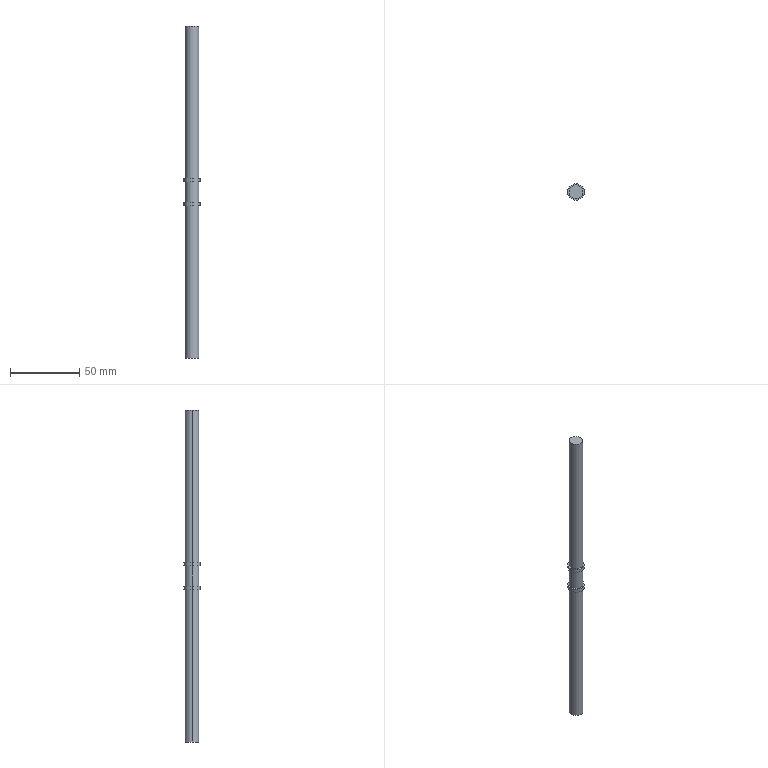Part | STEP file | Adjusting lead screw QY-1-16 | 1 solid | 16 faces | box 12 x 12 x 240 mm | volume 19022 mm3 | cylinder 10 | plane 6 | commonest cylinder face diameters 10 x6 12 x4
STEP:
#1=CARTESIAN_POINT('',(0.,0.,0.));
#2=DIRECTION('',(0.,0.,1.));
#3=DIRECTION('',(1.,0.,0.));
#4=AXIS2_PLACEMENT_3D('',#1,#2,#3);
#5=CARTESIAN_POINT('',(6.,0.,10.));
#6=VERTEX_POINT('',#5);
#7=CARTESIAN_POINT('',(-6.,0.,10.));
#8=VERTEX_POINT('',#7);
#9=CARTESIAN_POINT('',(0.,0.,10.));
#10=DIRECTION('',(0.,0.,1.));
#11=DIRECTION('',(1.,0.,0.));
#12=AXIS2_PLACEMENT_3D('',#9,#10,#11);
#13=CIRCLE('',#12,6.);
#14=CARTESIAN_POINT('',(0.,0.,10.));
#15=DIRECTION('',(0.,0.,-1.));
#16=DIRECTION('',(-1.,0.,0.));
#17=AXIS2_PLACEMENT_3D('',#14,#15,#16);
#18=CYLINDRICAL_SURFACE('',#17,6.);
#19=CARTESIAN_POINT('',(3.142,0.));
#20=DIRECTION('',(-1.,0.));
#21=VECTOR('',#20,1.);
#22=LINE('',#19,#21);
#23=(GEOMETRIC_REPRESENTATION_CONTEXT(2)PARAMETRIC_REPRESENTATION_CONTEXT()REPRESENTATION_CONTEXT('',''));
#24=DEFINITIONAL_REPRESENTATION('',(#22),#23);
#25=PCURVE('',#18,#24);
#26=CARTESIAN_POINT('',(0.,0.,10.));
#27=DIRECTION('',(0.,0.,1.));
#28=DIRECTION('',(1.,0.,0.));
#29=AXIS2_PLACEMENT_3D('',#26,#27,#28);
#30=PLANE('',#29);
#31=CARTESIAN_POINT('',(0.,0.));
#32=DIRECTION('',(1.,0.));
#33=AXIS2_PLACEMENT_2D('',#31,#32);
#34=CIRCLE('',#33,6.);
#35=(GEOMETRIC_REPRESENTATION_CONTEXT(2)PARAMETRIC_REPRESENTATION_CONTEXT()REPRESENTATION_CONTEXT('',''));
#36=DEFINITIONAL_REPRESENTATION('',(#34),#35);
#37=PCURVE('',#30,#36);
#38=SURFACE_CURVE('',#13,(#25,#37),.PCURVE_S1.);
#39=EDGE_CURVE('',#6,#8,#38,.T.);
#40=ORIENTED_EDGE('',*,*,#39,.F.);
#41=CARTESIAN_POINT('',(6.,0.,7.5));
#42=VERTEX_POINT('',#41);
#43=CARTESIAN_POINT('',(6.,0.,10.));
#44=DIRECTION('',(0.,0.,-1.));
#45=VECTOR('',#44,1.);
#46=LINE('',#43,#45);
#47=CARTESIAN_POINT('',(3.142,0.));
#48=DIRECTION('',(0.,1.));
#49=VECTOR('',#48,1.);
#50=LINE('',#47,#49);
#51=(GEOMETRIC_REPRESENTATION_CONTEXT(2)PARAMETRIC_REPRESENTATION_CONTEXT()REPRESENTATION_CONTEXT('',''));
#52=DEFINITIONAL_REPRESENTATION('',(#50),#51);
#53=PCURVE('',#18,#52);
#54=CARTESIAN_POINT('',(0.,0.,10.));
#55=DIRECTION('',(0.,0.,-1.));
#56=DIRECTION('',(-1.,0.,0.));
#57=AXIS2_PLACEMENT_3D('',#54,#55,#56);
#58=CYLINDRICAL_SURFACE('',#57,6.);
#59=CARTESIAN_POINT('',(3.142,0.));
#60=DIRECTION('',(0.,1.));
#61=VECTOR('',#60,1.);
#62=LINE('',#59,#61);
#63=(GEOMETRIC_REPRESENTATION_CONTEXT(2)PARAMETRIC_REPRESENTATION_CONTEXT()REPRESENTATION_CONTEXT('',''));
#64=DEFINITIONAL_REPRESENTATION('',(#62),#63);
#65=PCURVE('',#58,#64);
#66=SURFACE_CURVE('',#46,(#53,#65),.PCURVE_S1.);
#67=EDGE_CURVE('',#6,#42,#66,.T.);
#68=ORIENTED_EDGE('',*,*,#67,.T.);
#69=CARTESIAN_POINT('',(-6.,0.,7.5));
#70=VERTEX_POINT('',#69);
#71=CARTESIAN_POINT('',(0.,0.,7.5));
#72=DIRECTION('',(0.,0.,1.));
#73=DIRECTION('',(1.,0.,0.));
#74=AXIS2_PLACEMENT_3D('',#71,#72,#73);
#75=CIRCLE('',#74,6.);
#76=CARTESIAN_POINT('',(3.142,2.5));
#77=DIRECTION('',(-1.,0.));
#78=VECTOR('',#77,1.);
#79=LINE('',#76,#78);
#80=(GEOMETRIC_REPRESENTATION_CONTEXT(2)PARAMETRIC_REPRESENTATION_CONTEXT()REPRESENTATION_CONTEXT('',''));
#81=DEFINITIONAL_REPRESENTATION('',(#79),#80);
#82=PCURVE('',#18,#81);
#83=CARTESIAN_POINT('',(0.,0.,7.5));
#84=DIRECTION('',(0.,0.,1.));
#85=DIRECTION('',(1.,0.,0.));
#86=AXIS2_PLACEMENT_3D('',#83,#84,#85);
#87=PLANE('',#86);
#88=CARTESIAN_POINT('',(0.,0.));
#89=DIRECTION('',(1.,0.));
#90=AXIS2_PLACEMENT_2D('',#88,#89);
#91=CIRCLE('',#90,6.);
#92=(GEOMETRIC_REPRESENTATION_CONTEXT(2)PARAMETRIC_REPRESENTATION_CONTEXT()REPRESENTATION_CONTEXT('',''));
#93=DEFINITIONAL_REPRESENTATION('',(#91),#92);
#94=PCURVE('',#87,#93);
#95=SURFACE_CURVE('',#75,(#82,#94),.PCURVE_S1.);
#96=EDGE_CURVE('',#42,#70,#95,.T.);
#97=ORIENTED_EDGE('',*,*,#96,.T.);
#98=CARTESIAN_POINT('',(-6.,0.,10.));
#99=DIRECTION('',(0.,0.,-1.));
#100=VECTOR('',#99,1.);
#101=LINE('',#98,#100);
#102=CARTESIAN_POINT('',(0.,0.));
#103=DIRECTION('',(0.,1.));
#104=VECTOR('',#103,1.);
#105=LINE('',#102,#104);
#106=(GEOMETRIC_REPRESENTATION_CONTEXT(2)PARAMETRIC_REPRESENTATION_CONTEXT()REPRESENTATION_CONTEXT('',''));
#107=DEFINITIONAL_REPRESENTATION('',(#105),#106);
#108=PCURVE('',#18,#107);
#109=CARTESIAN_POINT('',(6.283,0.));
#110=DIRECTION('',(0.,1.));
#111=VECTOR('',#110,1.);
#112=LINE('',#109,#111);
#113=(GEOMETRIC_REPRESENTATION_CONTEXT(2)PARAMETRIC_REPRESENTATION_CONTEXT()REPRESENTATION_CONTEXT('',''));
#114=DEFINITIONAL_REPRESENTATION('',(#112),#113);
#115=PCURVE('',#58,#114);
#116=SURFACE_CURVE('',#101,(#108,#115),.PCURVE_S1.);
#117=EDGE_CURVE('',#8,#70,#116,.T.);
#118=ORIENTED_EDGE('',*,*,#117,.F.);
#119=EDGE_LOOP('',(#40,#68,#97,#118));
#120=FACE_BOUND('',#119,.T.);
#121=ADVANCED_FACE('',(#120),#18,.T.);
#122=CARTESIAN_POINT('',(5.,0.,120.));
#123=VERTEX_POINT('',#122);
#124=CARTESIAN_POINT('',(-5.,0.,120.));
#125=VERTEX_POINT('',#124);
#126=CARTESIAN_POINT('',(0.,0.,120.));
#127=DIRECTION('',(0.,0.,1.));
#128=DIRECTION('',(1.,0.,0.));
#129=AXIS2_PLACEMENT_3D('',#126,#127,#128);
#130=CIRCLE('',#129,5.);
#131=CARTESIAN_POINT('',(0.,0.,120.));
#132=DIRECTION('',(0.,0.,-1.));
#133=DIRECTION('',(-1.,0.,0.));
#134=AXIS2_PLACEMENT_3D('',#131,#132,#133);
#135=CYLINDRICAL_SURFACE('',#134,5.);
#136=CARTESIAN_POINT('',(3.142,0.));
#137=DIRECTION('',(-1.,0.));
#138=VECTOR('',#137,1.);
#139=LINE('',#136,#138);
#140=(GEOMETRIC_REPRESENTATION_CONTEXT(2)PARAMETRIC_REPRESENTATION_CONTEXT()REPRESENTATION_CONTEXT('',''));
#141=DEFINITIONAL_REPRESENTATION('',(#139),#140);
#142=PCURVE('',#135,#141);
#143=CARTESIAN_POINT('',(0.,0.,120.));
#144=DIRECTION('',(0.,0.,1.));
#145=DIRECTION('',(1.,0.,0.));
#146=AXIS2_PLACEMENT_3D('',#143,#144,#145);
#147=PLANE('',#146);
#148=CARTESIAN_POINT('',(0.,0.));
#149=DIRECTION('',(1.,0.));
#150=AXIS2_PLACEMENT_2D('',#148,#149);
#151=CIRCLE('',#150,5.);
#152=(GEOMETRIC_REPRESENTATION_CONTEXT(2)PARAMETRIC_REPRESENTATION_CONTEXT()REPRESENTATION_CONTEXT('',''));
#153=DEFINITIONAL_REPRESENTATION('',(#151),#152);
#154=PCURVE('',#147,#153);
#155=SURFACE_CURVE('',#130,(#142,#154),.PCURVE_S1.);
#156=EDGE_CURVE('',#123,#125,#155,.T.);
#157=ORIENTED_EDGE('',*,*,#156,.F.);
#158=CARTESIAN_POINT('',(5.,0.,10.));
#159=VERTEX_POINT('',#158);
#160=CARTESIAN_POINT('',(5.,0.,120.));
#161=DIRECTION('',(0.,0.,-1.));
#162=VECTOR('',#161,1.);
#163=LINE('',#160,#162);
#164=CARTESIAN_POINT('',(3.142,0.));
#165=DIRECTION('',(0.,1.));
#166=VECTOR('',#165,1.);
#167=LINE('',#164,#166);
#168=(GEOMETRIC_REPRESENTATION_CONTEXT(2)PARAMETRIC_REPRESENTATION_CONTEXT()REPRESENTATION_CONTEXT('',''));
#169=DEFINITIONAL_REPRESENTATION('',(#167),#168);
#170=PCURVE('',#135,#169);
#171=CARTESIAN_POINT('',(0.,0.,120.));
#172=DIRECTION('',(0.,0.,-1.));
#173=DIRECTION('',(-1.,0.,0.));
#174=AXIS2_PLACEMENT_3D('',#171,#172,#173);
#175=CYLINDRICAL_SURFACE('',#174,5.);
#176=CARTESIAN_POINT('',(3.142,0.));
#177=DIRECTION('',(0.,1.));
#178=VECTOR('',#177,1.);
#179=LINE('',#176,#178);
#180=(GEOMETRIC_REPRESENTATION_CONTEXT(2)PARAMETRIC_REPRESENTATION_CONTEXT()REPRESENTATION_CONTEXT('',''));
#181=DEFINITIONAL_REPRESENTATION('',(#179),#180);
#182=PCURVE('',#175,#181);
#183=SURFACE_CURVE('',#163,(#170,#182),.PCURVE_S1.);
#184=EDGE_CURVE('',#123,#159,#183,.T.);
#185=ORIENTED_EDGE('',*,*,#184,.T.);
#186=CARTESIAN_POINT('',(-5.,0.,10.));
#187=VERTEX_POINT('',#186);
#188=CARTESIAN_POINT('',(0.,0.,10.));
#189=DIRECTION('',(0.,0.,1.));
#190=DIRECTION('',(1.,0.,0.));
#191=AXIS2_PLACEMENT_3D('',#188,#189,#190);
#192=CIRCLE('',#191,5.);
#193=CARTESIAN_POINT('',(3.142,110.));
#194=DIRECTION('',(-1.,0.));
#195=VECTOR('',#194,1.);
#196=LINE('',#193,#195);
#197=(GEOMETRIC_REPRESENTATION_CONTEXT(2)PARAMETRIC_REPRESENTATION_CONTEXT()REPRESENTATION_CONTEXT('',''));
#198=DEFINITIONAL_REPRESENTATION('',(#196),#197);
#199=PCURVE('',#135,#198);
#200=CARTESIAN_POINT('',(0.,0.));
#201=DIRECTION('',(1.,0.));
#202=AXIS2_PLACEMENT_2D('',#200,#201);
#203=CIRCLE('',#202,5.);
#204=(GEOMETRIC_REPRESENTATION_CONTEXT(2)PARAMETRIC_REPRESENTATION_CONTEXT()REPRESENTATION_CONTEXT('',''));
#205=DEFINITIONAL_REPRESENTATION('',(#203),#204);
#206=PCURVE('',#30,#205);
#207=SURFACE_CURVE('',#192,(#199,#206),.PCURVE_S1.);
#208=EDGE_CURVE('',#159,#187,#207,.T.);
#209=ORIENTED_EDGE('',*,*,#208,.T.);
#210=CARTESIAN_POINT('',(-5.,0.,120.));
#211=DIRECTION('',(0.,0.,-1.));
#212=VECTOR('',#211,1.);
#213=LINE('',#210,#212);
#214=CARTESIAN_POINT('',(0.,0.));
#215=DIRECTION('',(0.,1.));
#216=VECTOR('',#215,1.);
#217=LINE('',#214,#216);
#218=(GEOMETRIC_REPRESENTATION_CONTEXT(2)PARAMETRIC_REPRESENTATION_CONTEXT()REPRESENTATION_CONTEXT('',''));
#219=DEFINITIONAL_REPRESENTATION('',(#217),#218);
#220=PCURVE('',#135,#219);
#221=CARTESIAN_POINT('',(6.283,0.));
#222=DIRECTION('',(0.,1.));
#223=VECTOR('',#222,1.);
#224=LINE('',#221,#223);
#225=(GEOMETRIC_REPRESENTATION_CONTEXT(2)PARAMETRIC_REPRESENTATION_CONTEXT()REPRESENTATION_CONTEXT('',''));
#226=DEFINITIONAL_REPRESENTATION('',(#224),#225);
#227=PCURVE('',#175,#226);
#228=SURFACE_CURVE('',#213,(#220,#227),.PCURVE_S1.);
#229=EDGE_CURVE('',#125,#187,#228,.T.);
#230=ORIENTED_EDGE('',*,*,#229,.F.);
#231=EDGE_LOOP('',(#157,#185,#209,#230));
#232=FACE_BOUND('',#231,.T.);
#233=ADVANCED_FACE('',(#232),#135,.T.);
#234=CARTESIAN_POINT('',(5.,0.,-7.5));
#235=VERTEX_POINT('',#234);
#236=CARTESIAN_POINT('',(-5.,0.,-7.5));
#237=VERTEX_POINT('',#236);
#238=CARTESIAN_POINT('',(0.,0.,-7.5));
#239=DIRECTION('',(0.,0.,1.));
#240=DIRECTION('',(1.,0.,0.));
#241=AXIS2_PLACEMENT_3D('',#238,#239,#240);
#242=CIRCLE('',#241,5.);
#243=CARTESIAN_POINT('',(0.,0.,-7.5));
#244=DIRECTION('',(0.,0.,1.));
#245=DIRECTION('',(1.,0.,0.));
#246=AXIS2_PLACEMENT_3D('',#243,#244,#245);
#247=CYLINDRICAL_SURFACE('',#246,5.);
#248=CARTESIAN_POINT('',(0.,0.));
#249=DIRECTION('',(1.,0.));
#250=VECTOR('',#249,1.);
#251=LINE('',#248,#250);
#252=(GEOMETRIC_REPRESENTATION_CONTEXT(2)PARAMETRIC_REPRESENTATION_CONTEXT()REPRESENTATION_CONTEXT('',''));
#253=DEFINITIONAL_REPRESENTATION('',(#251),#252);
#254=PCURVE('',#247,#253);
#255=CARTESIAN_POINT('',(0.,0.,-7.5));
#256=DIRECTION('',(0.,0.,1.));
#257=DIRECTION('',(1.,0.,0.));
#258=AXIS2_PLACEMENT_3D('',#255,#256,#257);
#259=PLANE('',#258);
#260=CARTESIAN_POINT('',(0.,0.));
#261=DIRECTION('',(1.,0.));
#262=AXIS2_PLACEMENT_2D('',#260,#261);
#263=CIRCLE('',#262,5.);
#264=(GEOMETRIC_REPRESENTATION_CONTEXT(2)PARAMETRIC_REPRESENTATION_CONTEXT()REPRESENTATION_CONTEXT('',''));
#265=DEFINITIONAL_REPRESENTATION('',(#263),#264);
#266=PCURVE('',#259,#265);
#267=SURFACE_CURVE('',#242,(#254,#266),.PCURVE_S1.);
#268=EDGE_CURVE('',#235,#237,#267,.T.);
#269=ORIENTED_EDGE('',*,*,#268,.T.);
#270=CARTESIAN_POINT('',(-5.,0.,7.5));
#271=VERTEX_POINT('',#270);
#272=CARTESIAN_POINT('',(-5.,0.,-7.5));
#273=DIRECTION('',(0.,0.,1.));
#274=VECTOR('',#273,1.);
#275=LINE('',#272,#274);
#276=CARTESIAN_POINT('',(3.142,0.));
#277=DIRECTION('',(0.,1.));
#278=VECTOR('',#277,1.);
#279=LINE('',#276,#278);
#280=(GEOMETRIC_REPRESENTATION_CONTEXT(2)PARAMETRIC_REPRESENTATION_CONTEXT()REPRESENTATION_CONTEXT('',''));
#281=DEFINITIONAL_REPRESENTATION('',(#279),#280);
#282=PCURVE('',#247,#281);
#283=CARTESIAN_POINT('',(0.,0.,-7.5));
#284=DIRECTION('',(0.,0.,1.));
#285=DIRECTION('',(1.,0.,0.));
#286=AXIS2_PLACEMENT_3D('',#283,#284,#285);
#287=CYLINDRICAL_SURFACE('',#286,5.);
#288=CARTESIAN_POINT('',(3.142,0.));
#289=DIRECTION('',(0.,1.));
#290=VECTOR('',#289,1.);
#291=LINE('',#288,#290);
#292=(GEOMETRIC_REPRESENTATION_CONTEXT(2)PARAMETRIC_REPRESENTATION_CONTEXT()REPRESENTATION_CONTEXT('',''));
#293=DEFINITIONAL_REPRESENTATION('',(#291),#292);
#294=PCURVE('',#287,#293);
#295=SURFACE_CURVE('',#275,(#282,#294),.PCURVE_S1.);
#296=EDGE_CURVE('',#237,#271,#295,.T.);
#297=ORIENTED_EDGE('',*,*,#296,.T.);
#298=CARTESIAN_POINT('',(5.,0.,7.5));
#299=VERTEX_POINT('',#298);
#300=CARTESIAN_POINT('',(0.,0.,7.5));
#301=DIRECTION('',(0.,0.,1.));
#302=DIRECTION('',(1.,0.,0.));
#303=AXIS2_PLACEMENT_3D('',#300,#301,#302);
#304=CIRCLE('',#303,5.);
#305=CARTESIAN_POINT('',(0.,15.));
#306=DIRECTION('',(1.,0.));
#307=VECTOR('',#306,1.);
#308=LINE('',#305,#307);
#309=(GEOMETRIC_REPRESENTATION_CONTEXT(2)PARAMETRIC_REPRESENTATION_CONTEXT()REPRESENTATION_CONTEXT('',''));
#310=DEFINITIONAL_REPRESENTATION('',(#308),#309);
#311=PCURVE('',#247,#310);
#312=CARTESIAN_POINT('',(0.,0.));
#313=DIRECTION('',(1.,0.));
#314=AXIS2_PLACEMENT_2D('',#312,#313);
#315=CIRCLE('',#314,5.);
#316=(GEOMETRIC_REPRESENTATION_CONTEXT(2)PARAMETRIC_REPRESENTATION_CONTEXT()REPRESENTATION_CONTEXT('',''));
#317=DEFINITIONAL_REPRESENTATION('',(#315),#316);
#318=PCURVE('',#87,#317);
#319=SURFACE_CURVE('',#304,(#311,#318),.PCURVE_S1.);
#320=EDGE_CURVE('',#299,#271,#319,.T.);
#321=ORIENTED_EDGE('',*,*,#320,.F.);
#322=CARTESIAN_POINT('',(5.,0.,-7.5));
#323=DIRECTION('',(0.,0.,1.));
#324=VECTOR('',#323,1.);
#325=LINE('',#322,#324);
#326=CARTESIAN_POINT('',(0.,0.));
#327=DIRECTION('',(0.,1.));
#328=VECTOR('',#327,1.);
#329=LINE('',#326,#328);
#330=(GEOMETRIC_REPRESENTATION_CONTEXT(2)PARAMETRIC_REPRESENTATION_CONTEXT()REPRESENTATION_CONTEXT('',''));
#331=DEFINITIONAL_REPRESENTATION('',(#329),#330);
#332=PCURVE('',#247,#331);
#333=CARTESIAN_POINT('',(6.283,0.));
#334=DIRECTION('',(0.,1.));
#335=VECTOR('',#334,1.);
#336=LINE('',#333,#335);
#337=(GEOMETRIC_REPRESENTATION_CONTEXT(2)PARAMETRIC_REPRESENTATION_CONTEXT()REPRESENTATION_CONTEXT('',''));
#338=DEFINITIONAL_REPRESENTATION('',(#336),#337);
#339=PCURVE('',#287,#338);
#340=SURFACE_CURVE('',#325,(#332,#339),.PCURVE_S1.);
#341=EDGE_CURVE('',#235,#299,#340,.T.);
#342=ORIENTED_EDGE('',*,*,#341,.F.);
#343=EDGE_LOOP('',(#269,#297,#321,#342));
#344=FACE_BOUND('',#343,.T.);
#345=ADVANCED_FACE('',(#344),#247,.T.);
#346=CARTESIAN_POINT('',(5.,0.,-10.));
#347=VERTEX_POINT('',#346);
#348=CARTESIAN_POINT('',(-5.,0.,-10.));
#349=VERTEX_POINT('',#348);
#350=CARTESIAN_POINT('',(0.,0.,-10.));
#351=DIRECTION('',(0.,0.,1.));
#352=DIRECTION('',(1.,0.,0.));
#353=AXIS2_PLACEMENT_3D('',#350,#351,#352);
#354=CIRCLE('',#353,5.);
#355=CARTESIAN_POINT('',(0.,0.,120.));
#356=DIRECTION('',(0.,0.,-1.));
#357=DIRECTION('',(-1.,0.,0.));
#358=AXIS2_PLACEMENT_3D('',#355,#356,#357);
#359=CYLINDRICAL_SURFACE('',#358,5.);
#360=CARTESIAN_POINT('',(3.142,130.));
#361=DIRECTION('',(-1.,0.));
#362=VECTOR('',#361,1.);
#363=LINE('',#360,#362);
#364=(GEOMETRIC_REPRESENTATION_CONTEXT(2)PARAMETRIC_REPRESENTATION_CONTEXT()REPRESENTATION_CONTEXT('',''));
#365=DEFINITIONAL_REPRESENTATION('',(#363),#364);
#366=PCURVE('',#359,#365);
#367=CARTESIAN_POINT('',(0.,0.,-10.));
#368=DIRECTION('',(0.,0.,1.));
#369=DIRECTION('',(1.,0.,0.));
#370=AXIS2_PLACEMENT_3D('',#367,#368,#369);
#371=PLANE('',#370);
#372=CARTESIAN_POINT('',(0.,0.));
#373=DIRECTION('',(1.,0.));
#374=AXIS2_PLACEMENT_2D('',#372,#373);
#375=CIRCLE('',#374,5.);
#376=(GEOMETRIC_REPRESENTATION_CONTEXT(2)PARAMETRIC_REPRESENTATION_CONTEXT()REPRESENTATION_CONTEXT('',''));
#377=DEFINITIONAL_REPRESENTATION('',(#375),#376);
#378=PCURVE('',#371,#377);
#379=SURFACE_CURVE('',#354,(#366,#378),.PCURVE_S1.);
#380=EDGE_CURVE('',#347,#349,#379,.T.);
#381=ORIENTED_EDGE('',*,*,#380,.F.);
#382=CARTESIAN_POINT('',(5.,0.,-120.));
#383=VERTEX_POINT('',#382);
#384=CARTESIAN_POINT('',(5.,0.,120.));
#385=DIRECTION('',(0.,0.,-1.));
#386=VECTOR('',#385,1.);
#387=LINE('',#384,#386);
#388=CARTESIAN_POINT('',(3.142,0.));
#389=DIRECTION('',(0.,1.));
#390=VECTOR('',#389,1.);
#391=LINE('',#388,#390);
#392=(GEOMETRIC_REPRESENTATION_CONTEXT(2)PARAMETRIC_REPRESENTATION_CONTEXT()REPRESENTATION_CONTEXT('',''));
#393=DEFINITIONAL_REPRESENTATION('',(#391),#392);
#394=PCURVE('',#359,#393);
#395=CARTESIAN_POINT('',(0.,0.,120.));
#396=DIRECTION('',(0.,0.,-1.));
#397=DIRECTION('',(-1.,0.,0.));
#398=AXIS2_PLACEMENT_3D('',#395,#396,#397);
#399=CYLINDRICAL_SURFACE('',#398,5.);
#400=CARTESIAN_POINT('',(3.142,0.));
#401=DIRECTION('',(0.,1.));
#402=VECTOR('',#401,1.);
#403=LINE('',#400,#402);
#404=(GEOMETRIC_REPRESENTATION_CONTEXT(2)PARAMETRIC_REPRESENTATION_CONTEXT()REPRESENTATION_CONTEXT('',''));
#405=DEFINITIONAL_REPRESENTATION('',(#403),#404);
#406=PCURVE('',#399,#405);
#407=SURFACE_CURVE('',#387,(#394,#406),.PCURVE_S1.);
#408=EDGE_CURVE('',#347,#383,#407,.T.);
#409=ORIENTED_EDGE('',*,*,#408,.T.);
#410=CARTESIAN_POINT('',(-5.,0.,-120.));
#411=VERTEX_POINT('',#410);
#412=CARTESIAN_POINT('',(0.,0.,-120.));
#413=DIRECTION('',(0.,0.,1.));
#414=DIRECTION('',(1.,0.,0.));
#415=AXIS2_PLACEMENT_3D('',#412,#413,#414);
#416=CIRCLE('',#415,5.);
#417=CARTESIAN_POINT('',(3.142,240.));
#418=DIRECTION('',(-1.,0.));
#419=VECTOR('',#418,1.);
#420=LINE('',#417,#419);
#421=(GEOMETRIC_REPRESENTATION_CONTEXT(2)PARAMETRIC_REPRESENTATION_CONTEXT()REPRESENTATION_CONTEXT('',''));
#422=DEFINITIONAL_REPRESENTATION('',(#420),#421);
#423=PCURVE('',#359,#422);
#424=CARTESIAN_POINT('',(0.,0.,-120.));
#425=DIRECTION('',(0.,0.,1.));
#426=DIRECTION('',(1.,0.,0.));
#427=AXIS2_PLACEMENT_3D('',#424,#425,#426);
#428=PLANE('',#427);
#429=CARTESIAN_POINT('',(0.,0.));
#430=DIRECTION('',(1.,0.));
#431=AXIS2_PLACEMENT_2D('',#429,#430);
#432=CIRCLE('',#431,5.);
#433=(GEOMETRIC_REPRESENTATION_CONTEXT(2)PARAMETRIC_REPRESENTATION_CONTEXT()REPRESENTATION_CONTEXT('',''));
#434=DEFINITIONAL_REPRESENTATION('',(#432),#433);
#435=PCURVE('',#428,#434);
#436=SURFACE_CURVE('',#416,(#423,#435),.PCURVE_S1.);
#437=EDGE_CURVE('',#383,#411,#436,.T.);
#438=ORIENTED_EDGE('',*,*,#437,.T.);
#439=CARTESIAN_POINT('',(-5.,0.,120.));
#440=DIRECTION('',(0.,0.,-1.));
#441=VECTOR('',#440,1.);
#442=LINE('',#439,#441);
#443=CARTESIAN_POINT('',(0.,0.));
#444=DIRECTION('',(0.,1.));
#445=VECTOR('',#444,1.);
#446=LINE('',#443,#445);
#447=(GEOMETRIC_REPRESENTATION_CONTEXT(2)PARAMETRIC_REPRESENTATION_CONTEXT()REPRESENTATION_CONTEXT('',''));
#448=DEFINITIONAL_REPRESENTATION('',(#446),#447);
#449=PCURVE('',#359,#448);
#450=CARTESIAN_POINT('',(6.283,0.));
#451=DIRECTION('',(0.,1.));
#452=VECTOR('',#451,1.);
#453=LINE('',#450,#452);
#454=(GEOMETRIC_REPRESENTATION_CONTEXT(2)PARAMETRIC_REPRESENTATION_CONTEXT()REPRESENTATION_CONTEXT('',''));
#455=DEFINITIONAL_REPRESENTATION('',(#453),#454);
#456=PCURVE('',#399,#455);
#457=SURFACE_CURVE('',#442,(#449,#456),.PCURVE_S1.);
#458=EDGE_CURVE('',#349,#411,#457,.T.);
#459=ORIENTED_EDGE('',*,*,#458,.F.);
#460=EDGE_LOOP('',(#381,#409,#438,#459));
#461=FACE_BOUND('',#460,.T.);
#462=ADVANCED_FACE('',(#461),#359,.T.);
#463=CARTESIAN_POINT('',(6.,0.,-7.5));
#464=VERTEX_POINT('',#463);
#465=CARTESIAN_POINT('',(-6.,0.,-7.5));
#466=VERTEX_POINT('',#465);
#467=CARTESIAN_POINT('',(0.,0.,-7.5));
#468=DIRECTION('',(0.,0.,1.));
#469=DIRECTION('',(1.,0.,0.));
#470=AXIS2_PLACEMENT_3D('',#467,#468,#469);
#471=CIRCLE('',#470,6.);
#472=CARTESIAN_POINT('',(0.,0.,10.));
#473=DIRECTION('',(0.,0.,-1.));
#474=DIRECTION('',(-1.,0.,0.));
#475=AXIS2_PLACEMENT_3D('',#472,#473,#474);
#476=CYLINDRICAL_SURFACE('',#475,6.);
#477=CARTESIAN_POINT('',(3.142,17.5));
#478=DIRECTION('',(-1.,0.));
#479=VECTOR('',#478,1.);
#480=LINE('',#477,#479);
#481=(GEOMETRIC_REPRESENTATION_CONTEXT(2)PARAMETRIC_REPRESENTATION_CONTEXT()REPRESENTATION_CONTEXT('',''));
#482=DEFINITIONAL_REPRESENTATION('',(#480),#481);
#483=PCURVE('',#476,#482);
#484=CARTESIAN_POINT('',(0.,0.));
#485=DIRECTION('',(1.,0.));
#486=AXIS2_PLACEMENT_2D('',#484,#485);
#487=CIRCLE('',#486,6.);
#488=(GEOMETRIC_REPRESENTATION_CONTEXT(2)PARAMETRIC_REPRESENTATION_CONTEXT()REPRESENTATION_CONTEXT('',''));
#489=DEFINITIONAL_REPRESENTATION('',(#487),#488);
#490=PCURVE('',#259,#489);
#491=SURFACE_CURVE('',#471,(#483,#490),.PCURVE_S1.);
#492=EDGE_CURVE('',#464,#466,#491,.T.);
#493=ORIENTED_EDGE('',*,*,#492,.F.);
#494=CARTESIAN_POINT('',(6.,0.,-10.));
#495=VERTEX_POINT('',#494);
#496=CARTESIAN_POINT('',(6.,0.,10.));
#497=DIRECTION('',(0.,0.,-1.));
#498=VECTOR('',#497,1.);
#499=LINE('',#496,#498);
#500=CARTESIAN_POINT('',(3.142,0.));
#501=DIRECTION('',(0.,1.));
#502=VECTOR('',#501,1.);
#503=LINE('',#500,#502);
#504=(GEOMETRIC_REPRESENTATION_CONTEXT(2)PARAMETRIC_REPRESENTATION_CONTEXT()REPRESENTATION_CONTEXT('',''));
#505=DEFINITIONAL_REPRESENTATION('',(#503),#504);
#506=PCURVE('',#476,#505);
#507=CARTESIAN_POINT('',(0.,0.,10.));
#508=DIRECTION('',(0.,0.,-1.));
#509=DIRECTION('',(-1.,0.,0.));
#510=AXIS2_PLACEMENT_3D('',#507,#508,#509);
#511=CYLINDRICAL_SURFACE('',#510,6.);
#512=CARTESIAN_POINT('',(3.142,0.));
#513=DIRECTION('',(0.,1.));
#514=VECTOR('',#513,1.);
#515=LINE('',#512,#514);
#516=(GEOMETRIC_REPRESENTATION_CONTEXT(2)PARAMETRIC_REPRESENTATION_CONTEXT()REPRESENTATION_CONTEXT('',''));
#517=DEFINITIONAL_REPRESENTATION('',(#515),#516);
#518=PCURVE('',#511,#517);
#519=SURFACE_CURVE('',#499,(#506,#518),.PCURVE_S1.);
#520=EDGE_CURVE('',#464,#495,#519,.T.);
#521=ORIENTED_EDGE('',*,*,#520,.T.);
#522=CARTESIAN_POINT('',(-6.,0.,-10.));
#523=VERTEX_POINT('',#522);
#524=CARTESIAN_POINT('',(0.,0.,-10.));
#525=DIRECTION('',(0.,0.,1.));
#526=DIRECTION('',(1.,0.,0.));
#527=AXIS2_PLACEMENT_3D('',#524,#525,#526);
#528=CIRCLE('',#527,6.);
#529=CARTESIAN_POINT('',(3.142,20.));
#530=DIRECTION('',(-1.,0.));
#531=VECTOR('',#530,1.);
#532=LINE('',#529,#531);
#533=(GEOMETRIC_REPRESENTATION_CONTEXT(2)PARAMETRIC_REPRESENTATION_CONTEXT()REPRESENTATION_CONTEXT('',''));
#534=DEFINITIONAL_REPRESENTATION('',(#532),#533);
#535=PCURVE('',#476,#534);
#536=CARTESIAN_POINT('',(0.,0.));
#537=DIRECTION('',(1.,0.));
#538=AXIS2_PLACEMENT_2D('',#536,#537);
#539=CIRCLE('',#538,6.);
#540=(GEOMETRIC_REPRESENTATION_CONTEXT(2)PARAMETRIC_REPRESENTATION_CONTEXT()REPRESENTATION_CONTEXT('',''));
#541=DEFINITIONAL_REPRESENTATION('',(#539),#540);
#542=PCURVE('',#371,#541);
#543=SURFACE_CURVE('',#528,(#535,#542),.PCURVE_S1.);
#544=EDGE_CURVE('',#495,#523,#543,.T.);
#545=ORIENTED_EDGE('',*,*,#544,.T.);
#546=CARTESIAN_POINT('',(-6.,0.,10.));
#547=DIRECTION('',(0.,0.,-1.));
#548=VECTOR('',#547,1.);
#549=LINE('',#546,#548);
#550=CARTESIAN_POINT('',(0.,0.));
#551=DIRECTION('',(0.,1.));
#552=VECTOR('',#551,1.);
#553=LINE('',#550,#552);
#554=(GEOMETRIC_REPRESENTATION_CONTEXT(2)PARAMETRIC_REPRESENTATION_CONTEXT()REPRESENTATION_CONTEXT('',''));
#555=DEFINITIONAL_REPRESENTATION('',(#553),#554);
#556=PCURVE('',#476,#555);
#557=CARTESIAN_POINT('',(6.283,0.));
#558=DIRECTION('',(0.,1.));
#559=VECTOR('',#558,1.);
#560=LINE('',#557,#559);
#561=(GEOMETRIC_REPRESENTATION_CONTEXT(2)PARAMETRIC_REPRESENTATION_CONTEXT()REPRESENTATION_CONTEXT('',''));
#562=DEFINITIONAL_REPRESENTATION('',(#560),#561);
#563=PCURVE('',#511,#562);
#564=SURFACE_CURVE('',#549,(#556,#563),.PCURVE_S1.);
#565=EDGE_CURVE('',#466,#523,#564,.T.);
#566=ORIENTED_EDGE('',*,*,#565,.F.);
#567=EDGE_LOOP('',(#493,#521,#545,#566));
#568=FACE_BOUND('',#567,.T.);
#569=ADVANCED_FACE('',(#568),#476,.T.);
#570=ORIENTED_EDGE('',*,*,#520,.F.);
#571=CARTESIAN_POINT('',(0.,0.,-7.5));
#572=DIRECTION('',(0.,0.,1.));
#573=DIRECTION('',(1.,0.,0.));
#574=AXIS2_PLACEMENT_3D('',#571,#572,#573);
#575=CIRCLE('',#574,6.);
#576=CARTESIAN_POINT('',(9.425,17.5));
#577=DIRECTION('',(-1.,0.));
#578=VECTOR('',#577,1.);
#579=LINE('',#576,#578);
#580=(GEOMETRIC_REPRESENTATION_CONTEXT(2)PARAMETRIC_REPRESENTATION_CONTEXT()REPRESENTATION_CONTEXT('',''));
#581=DEFINITIONAL_REPRESENTATION('',(#579),#580);
#582=PCURVE('',#511,#581);
#583=CARTESIAN_POINT('',(0.,0.));
#584=DIRECTION('',(1.,0.));
#585=AXIS2_PLACEMENT_2D('',#583,#584);
#586=CIRCLE('',#585,6.);
#587=(GEOMETRIC_REPRESENTATION_CONTEXT(2)PARAMETRIC_REPRESENTATION_CONTEXT()REPRESENTATION_CONTEXT('',''));
#588=DEFINITIONAL_REPRESENTATION('',(#586),#587);
#589=PCURVE('',#259,#588);
#590=SURFACE_CURVE('',#575,(#582,#589),.PCURVE_S1.);
#591=EDGE_CURVE('',#466,#464,#590,.T.);
#592=ORIENTED_EDGE('',*,*,#591,.F.);
#593=ORIENTED_EDGE('',*,*,#565,.T.);
#594=CARTESIAN_POINT('',(0.,0.,-10.));
#595=DIRECTION('',(0.,0.,1.));
#596=DIRECTION('',(1.,0.,0.));
#597=AXIS2_PLACEMENT_3D('',#594,#595,#596);
#598=CIRCLE('',#597,6.);
#599=CARTESIAN_POINT('',(9.425,20.));
#600=DIRECTION('',(-1.,0.));
#601=VECTOR('',#600,1.);
#602=LINE('',#599,#601);
#603=(GEOMETRIC_REPRESENTATION_CONTEXT(2)PARAMETRIC_REPRESENTATION_CONTEXT()REPRESENTATION_CONTEXT('',''));
#604=DEFINITIONAL_REPRESENTATION('',(#602),#603);
#605=PCURVE('',#511,#604);
#606=CARTESIAN_POINT('',(0.,0.));
#607=DIRECTION('',(1.,0.));
#608=AXIS2_PLACEMENT_2D('',#606,#607);
#609=CIRCLE('',#608,6.);
#610=(GEOMETRIC_REPRESENTATION_CONTEXT(2)PARAMETRIC_REPRESENTATION_CONTEXT()REPRESENTATION_CONTEXT('',''));
#611=DEFINITIONAL_REPRESENTATION('',(#609),#610);
#612=PCURVE('',#371,#611);
#613=SURFACE_CURVE('',#598,(#605,#612),.PCURVE_S1.);
#614=EDGE_CURVE('',#523,#495,#613,.T.);
#615=ORIENTED_EDGE('',*,*,#614,.T.);
#616=EDGE_LOOP('',(#570,#592,#593,#615));
#617=FACE_BOUND('',#616,.T.);
#618=ADVANCED_FACE('',(#617),#511,.T.);
#619=CARTESIAN_POINT('',(0.,0.,-10.));
#620=DIRECTION('',(0.,0.,1.));
#621=DIRECTION('',(1.,0.,0.));
#622=AXIS2_PLACEMENT_3D('',#619,#620,#621);
#623=CIRCLE('',#622,5.);
#624=CARTESIAN_POINT('',(0.,0.));
#625=DIRECTION('',(1.,0.));
#626=AXIS2_PLACEMENT_2D('',#624,#625);
#627=CIRCLE('',#626,5.);
#628=(GEOMETRIC_REPRESENTATION_CONTEXT(2)PARAMETRIC_REPRESENTATION_CONTEXT()REPRESENTATION_CONTEXT('',''));
#629=DEFINITIONAL_REPRESENTATION('',(#627),#628);
#630=PCURVE('',#371,#629);
#631=CARTESIAN_POINT('',(9.425,130.));
#632=DIRECTION('',(-1.,0.));
#633=VECTOR('',#632,1.);
#634=LINE('',#631,#633);
#635=(GEOMETRIC_REPRESENTATION_CONTEXT(2)PARAMETRIC_REPRESENTATION_CONTEXT()REPRESENTATION_CONTEXT('',''));
#636=DEFINITIONAL_REPRESENTATION('',(#634),#635);
#637=PCURVE('',#399,#636);
#638=SURFACE_CURVE('',#623,(#630,#637),.PCURVE_S1.);
#639=EDGE_CURVE('',#349,#347,#638,.T.);
#640=ORIENTED_EDGE('',*,*,#639,.T.);
#641=ORIENTED_EDGE('',*,*,#380,.T.);
#642=EDGE_LOOP('',(#640,#641));
#643=FACE_BOUND('',#642,.T.);
#644=ORIENTED_EDGE('',*,*,#614,.F.);
#645=ORIENTED_EDGE('',*,*,#544,.F.);
#646=EDGE_LOOP('',(#644,#645));
#647=FACE_BOUND('',#646,.T.);
#648=ADVANCED_FACE('',(#643,#647),#371,.F.);
#649=CARTESIAN_POINT('',(0.,0.,-120.));
#650=DIRECTION('',(0.,0.,1.));
#651=DIRECTION('',(1.,0.,0.));
#652=AXIS2_PLACEMENT_3D('',#649,#650,#651);
#653=CIRCLE('',#652,5.);
#654=CARTESIAN_POINT('',(0.,0.));
#655=DIRECTION('',(1.,0.));
#656=AXIS2_PLACEMENT_2D('',#654,#655);
#657=CIRCLE('',#656,5.);
#658=(GEOMETRIC_REPRESENTATION_CONTEXT(2)PARAMETRIC_REPRESENTATION_CONTEXT()REPRESENTATION_CONTEXT('',''));
#659=DEFINITIONAL_REPRESENTATION('',(#657),#658);
#660=PCURVE('',#428,#659);
#661=CARTESIAN_POINT('',(9.425,240.));
#662=DIRECTION('',(-1.,0.));
#663=VECTOR('',#662,1.);
#664=LINE('',#661,#663);
#665=(GEOMETRIC_REPRESENTATION_CONTEXT(2)PARAMETRIC_REPRESENTATION_CONTEXT()REPRESENTATION_CONTEXT('',''));
#666=DEFINITIONAL_REPRESENTATION('',(#664),#665);
#667=PCURVE('',#399,#666);
#668=SURFACE_CURVE('',#653,(#660,#667),.PCURVE_S1.);
#669=EDGE_CURVE('',#411,#383,#668,.T.);
#670=ORIENTED_EDGE('',*,*,#669,.F.);
#671=ORIENTED_EDGE('',*,*,#437,.F.);
#672=EDGE_LOOP('',(#670,#671));
#673=FACE_BOUND('',#672,.T.);
#674=ADVANCED_FACE('',(#673),#428,.F.);
#675=ORIENTED_EDGE('',*,*,#408,.F.);
#676=ORIENTED_EDGE('',*,*,#639,.F.);
#677=ORIENTED_EDGE('',*,*,#458,.T.);
#678=ORIENTED_EDGE('',*,*,#669,.T.);
#679=EDGE_LOOP('',(#675,#676,#677,#678));
#680=FACE_BOUND('',#679,.T.);
#681=ADVANCED_FACE('',(#680),#399,.T.);
#682=ORIENTED_EDGE('',*,*,#268,.F.);
#683=CARTESIAN_POINT('',(0.,0.,-7.5));
#684=DIRECTION('',(0.,0.,1.));
#685=DIRECTION('',(1.,0.,0.));
#686=AXIS2_PLACEMENT_3D('',#683,#684,#685);
#687=CIRCLE('',#686,5.);
#688=CARTESIAN_POINT('',(0.,0.));
#689=DIRECTION('',(1.,0.));
#690=AXIS2_PLACEMENT_2D('',#688,#689);
#691=CIRCLE('',#690,5.);
#692=(GEOMETRIC_REPRESENTATION_CONTEXT(2)PARAMETRIC_REPRESENTATION_CONTEXT()REPRESENTATION_CONTEXT('',''));
#693=DEFINITIONAL_REPRESENTATION('',(#691),#692);
#694=PCURVE('',#259,#693);
#695=CARTESIAN_POINT('',(0.,0.));
#696=DIRECTION('',(1.,0.));
#697=VECTOR('',#696,1.);
#698=LINE('',#695,#697);
#699=(GEOMETRIC_REPRESENTATION_CONTEXT(2)PARAMETRIC_REPRESENTATION_CONTEXT()REPRESENTATION_CONTEXT('',''));
#700=DEFINITIONAL_REPRESENTATION('',(#698),#699);
#701=PCURVE('',#287,#700);
#702=SURFACE_CURVE('',#687,(#694,#701),.PCURVE_S1.);
#703=EDGE_CURVE('',#237,#235,#702,.T.);
#704=ORIENTED_EDGE('',*,*,#703,.F.);
#705=EDGE_LOOP('',(#682,#704));
#706=FACE_BOUND('',#705,.T.);
#707=ORIENTED_EDGE('',*,*,#591,.T.);
#708=ORIENTED_EDGE('',*,*,#492,.T.);
#709=EDGE_LOOP('',(#707,#708));
#710=FACE_BOUND('',#709,.T.);
#711=ADVANCED_FACE('',(#706,#710),#259,.T.);
#712=ORIENTED_EDGE('',*,*,#320,.T.);
#713=CARTESIAN_POINT('',(0.,0.,7.5));
#714=DIRECTION('',(0.,0.,1.));
#715=DIRECTION('',(1.,0.,0.));
#716=AXIS2_PLACEMENT_3D('',#713,#714,#715);
#717=CIRCLE('',#716,5.);
#718=CARTESIAN_POINT('',(0.,0.));
#719=DIRECTION('',(1.,0.));
#720=AXIS2_PLACEMENT_2D('',#718,#719);
#721=CIRCLE('',#720,5.);
#722=(GEOMETRIC_REPRESENTATION_CONTEXT(2)PARAMETRIC_REPRESENTATION_CONTEXT()REPRESENTATION_CONTEXT('',''));
#723=DEFINITIONAL_REPRESENTATION('',(#721),#722);
#724=PCURVE('',#87,#723);
#725=CARTESIAN_POINT('',(0.,15.));
#726=DIRECTION('',(1.,0.));
#727=VECTOR('',#726,1.);
#728=LINE('',#725,#727);
#729=(GEOMETRIC_REPRESENTATION_CONTEXT(2)PARAMETRIC_REPRESENTATION_CONTEXT()REPRESENTATION_CONTEXT('',''));
#730=DEFINITIONAL_REPRESENTATION('',(#728),#729);
#731=PCURVE('',#287,#730);
#732=SURFACE_CURVE('',#717,(#724,#731),.PCURVE_S1.);
#733=EDGE_CURVE('',#271,#299,#732,.T.);
#734=ORIENTED_EDGE('',*,*,#733,.T.);
#735=EDGE_LOOP('',(#712,#734));
#736=FACE_BOUND('',#735,.T.);
#737=CARTESIAN_POINT('',(0.,0.,7.5));
#738=DIRECTION('',(0.,0.,1.));
#739=DIRECTION('',(1.,0.,0.));
#740=AXIS2_PLACEMENT_3D('',#737,#738,#739);
#741=CIRCLE('',#740,6.);
#742=CARTESIAN_POINT('',(0.,0.));
#743=DIRECTION('',(1.,0.));
#744=AXIS2_PLACEMENT_2D('',#742,#743);
#745=CIRCLE('',#744,6.);
#746=(GEOMETRIC_REPRESENTATION_CONTEXT(2)PARAMETRIC_REPRESENTATION_CONTEXT()REPRESENTATION_CONTEXT('',''));
#747=DEFINITIONAL_REPRESENTATION('',(#745),#746);
#748=PCURVE('',#87,#747);
#749=CARTESIAN_POINT('',(9.425,2.5));
#750=DIRECTION('',(-1.,0.));
#751=VECTOR('',#750,1.);
#752=LINE('',#749,#751);
#753=(GEOMETRIC_REPRESENTATION_CONTEXT(2)PARAMETRIC_REPRESENTATION_CONTEXT()REPRESENTATION_CONTEXT('',''));
#754=DEFINITIONAL_REPRESENTATION('',(#752),#753);
#755=PCURVE('',#58,#754);
#756=SURFACE_CURVE('',#741,(#748,#755),.PCURVE_S1.);
#757=EDGE_CURVE('',#70,#42,#756,.T.);
#758=ORIENTED_EDGE('',*,*,#757,.F.);
#759=ORIENTED_EDGE('',*,*,#96,.F.);
#760=EDGE_LOOP('',(#758,#759));
#761=FACE_BOUND('',#760,.T.);
#762=ADVANCED_FACE('',(#736,#761),#87,.F.);
#763=ORIENTED_EDGE('',*,*,#296,.F.);
#764=ORIENTED_EDGE('',*,*,#703,.T.);
#765=ORIENTED_EDGE('',*,*,#341,.T.);
#766=ORIENTED_EDGE('',*,*,#733,.F.);
#767=EDGE_LOOP('',(#763,#764,#765,#766));
#768=FACE_BOUND('',#767,.T.);
#769=ADVANCED_FACE('',(#768),#287,.T.);
#770=CARTESIAN_POINT('',(0.,0.,120.));
#771=DIRECTION('',(0.,0.,1.));
#772=DIRECTION('',(1.,0.,0.));
#773=AXIS2_PLACEMENT_3D('',#770,#771,#772);
#774=CIRCLE('',#773,5.);
#775=CARTESIAN_POINT('',(0.,0.));
#776=DIRECTION('',(1.,0.));
#777=AXIS2_PLACEMENT_2D('',#775,#776);
#778=CIRCLE('',#777,5.);
#779=(GEOMETRIC_REPRESENTATION_CONTEXT(2)PARAMETRIC_REPRESENTATION_CONTEXT()REPRESENTATION_CONTEXT('',''));
#780=DEFINITIONAL_REPRESENTATION('',(#778),#779);
#781=PCURVE('',#147,#780);
#782=CARTESIAN_POINT('',(9.425,0.));
#783=DIRECTION('',(-1.,0.));
#784=VECTOR('',#783,1.);
#785=LINE('',#782,#784);
#786=(GEOMETRIC_REPRESENTATION_CONTEXT(2)PARAMETRIC_REPRESENTATION_CONTEXT()REPRESENTATION_CONTEXT('',''));
#787=DEFINITIONAL_REPRESENTATION('',(#785),#786);
#788=PCURVE('',#175,#787);
#789=SURFACE_CURVE('',#774,(#781,#788),.PCURVE_S1.);
#790=EDGE_CURVE('',#125,#123,#789,.T.);
#791=ORIENTED_EDGE('',*,*,#790,.T.);
#792=ORIENTED_EDGE('',*,*,#156,.T.);
#793=EDGE_LOOP('',(#791,#792));
#794=FACE_BOUND('',#793,.T.);
#795=ADVANCED_FACE('',(#794),#147,.T.);
#796=ORIENTED_EDGE('',*,*,#184,.F.);
#797=ORIENTED_EDGE('',*,*,#790,.F.);
#798=ORIENTED_EDGE('',*,*,#229,.T.);
#799=CARTESIAN_POINT('',(0.,0.,10.));
#800=DIRECTION('',(0.,0.,1.));
#801=DIRECTION('',(1.,0.,0.));
#802=AXIS2_PLACEMENT_3D('',#799,#800,#801);
#803=CIRCLE('',#802,5.);
#804=CARTESIAN_POINT('',(9.425,110.));
#805=DIRECTION('',(-1.,0.));
#806=VECTOR('',#805,1.);
#807=LINE('',#804,#806);
#808=(GEOMETRIC_REPRESENTATION_CONTEXT(2)PARAMETRIC_REPRESENTATION_CONTEXT()REPRESENTATION_CONTEXT('',''));
#809=DEFINITIONAL_REPRESENTATION('',(#807),#808);
#810=PCURVE('',#175,#809);
#811=CARTESIAN_POINT('',(0.,0.));
#812=DIRECTION('',(1.,0.));
#813=AXIS2_PLACEMENT_2D('',#811,#812);
#814=CIRCLE('',#813,5.);
#815=(GEOMETRIC_REPRESENTATION_CONTEXT(2)PARAMETRIC_REPRESENTATION_CONTEXT()REPRESENTATION_CONTEXT('',''));
#816=DEFINITIONAL_REPRESENTATION('',(#814),#815);
#817=PCURVE('',#30,#816);
#818=SURFACE_CURVE('',#803,(#810,#817),.PCURVE_S1.);
#819=EDGE_CURVE('',#187,#159,#818,.T.);
#820=ORIENTED_EDGE('',*,*,#819,.T.);
#821=EDGE_LOOP('',(#796,#797,#798,#820));
#822=FACE_BOUND('',#821,.T.);
#823=ADVANCED_FACE('',(#822),#175,.T.);
#824=ORIENTED_EDGE('',*,*,#819,.F.);
#825=ORIENTED_EDGE('',*,*,#208,.F.);
#826=EDGE_LOOP('',(#824,#825));
#827=FACE_BOUND('',#826,.T.);
#828=CARTESIAN_POINT('',(0.,0.,10.));
#829=DIRECTION('',(0.,0.,1.));
#830=DIRECTION('',(1.,0.,0.));
#831=AXIS2_PLACEMENT_3D('',#828,#829,#830);
#832=CIRCLE('',#831,6.);
#833=CARTESIAN_POINT('',(0.,0.));
#834=DIRECTION('',(1.,0.));
#835=AXIS2_PLACEMENT_2D('',#833,#834);
#836=CIRCLE('',#835,6.);
#837=(GEOMETRIC_REPRESENTATION_CONTEXT(2)PARAMETRIC_REPRESENTATION_CONTEXT()REPRESENTATION_CONTEXT('',''));
#838=DEFINITIONAL_REPRESENTATION('',(#836),#837);
#839=PCURVE('',#30,#838);
#840=CARTESIAN_POINT('',(9.425,0.));
#841=DIRECTION('',(-1.,0.));
#842=VECTOR('',#841,1.);
#843=LINE('',#840,#842);
#844=(GEOMETRIC_REPRESENTATION_CONTEXT(2)PARAMETRIC_REPRESENTATION_CONTEXT()REPRESENTATION_CONTEXT('',''));
#845=DEFINITIONAL_REPRESENTATION('',(#843),#844);
#846=PCURVE('',#58,#845);
#847=SURFACE_CURVE('',#832,(#839,#846),.PCURVE_S1.);
#848=EDGE_CURVE('',#8,#6,#847,.T.);
#849=ORIENTED_EDGE('',*,*,#848,.T.);
#850=ORIENTED_EDGE('',*,*,#39,.T.);
#851=EDGE_LOOP('',(#849,#850));
#852=FACE_BOUND('',#851,.T.);
#853=ADVANCED_FACE('',(#827,#852),#30,.T.);
#854=ORIENTED_EDGE('',*,*,#67,.F.);
#855=ORIENTED_EDGE('',*,*,#848,.F.);
#856=ORIENTED_EDGE('',*,*,#117,.T.);
#857=ORIENTED_EDGE('',*,*,#757,.T.);
#858=EDGE_LOOP('',(#854,#855,#856,#857));
#859=FACE_BOUND('',#858,.T.);
#860=ADVANCED_FACE('',(#859),#58,.T.);
#861=CLOSED_SHELL('',(#121,#233,#345,#462,#569,#618,#648,#674,#681,#711,#762,#769,#795,#823,#853,#860));
#862=MANIFOLD_SOLID_BREP('',#861);
#863=(LENGTH_UNIT()NAMED_UNIT(*)SI_UNIT(.MILLI.,.METRE.));
#864=UNCERTAINTY_MEASURE_WITH_UNIT(LENGTH_MEASURE(0.0000001),#863,'','');
#865=(NAMED_UNIT(*)PLANE_ANGLE_UNIT()SI_UNIT($,.RADIAN.));
#866=(NAMED_UNIT(*)SI_UNIT($,.STERADIAN.)SOLID_ANGLE_UNIT());
#867=(GEOMETRIC_REPRESENTATION_CONTEXT(3)GLOBAL_UNCERTAINTY_ASSIGNED_CONTEXT((#864))GLOBAL_UNIT_ASSIGNED_CONTEXT((#863,#865,#866))REPRESENTATION_CONTEXT('',''));
#868=ADVANCED_BREP_SHAPE_REPRESENTATION('',(#4,#862),#867);